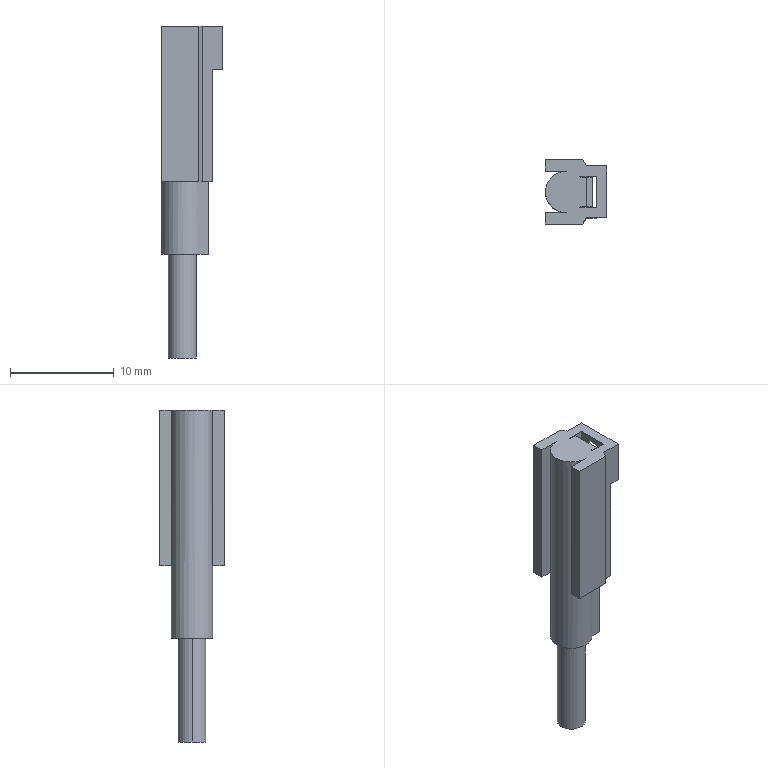Part | SolidWorks | features ICE 8, RefAxis 3, 3DProfileFeature 1, Extrusion 1 | 1 solid | 51 faces | box 5.9 x 6.2 x 32 mm | volume 553.468 mm3 | plane 37 | cylinder 14 | commonest cylinder face diameters 0.8 x4 2.1 x3 2.5 x2 2.7 x2 2.9 x2 4 x1
STEP:
#1=CARTESIAN_POINT('',(1.35,0.,-32.));
#2=VERTEX_POINT('',#1);
#3=CARTESIAN_POINT('',(-1.35,0.,-32.));
#4=VERTEX_POINT('',#3);
#5=CARTESIAN_POINT('',(0.,0.,-32.));
#6=DIRECTION('',(0.,0.,1.));
#7=DIRECTION('',(1.,0.,0.));
#8=AXIS2_PLACEMENT_3D('',#5,#6,#7);
#9=CIRCLE('',#8,1.35);
#10=EDGE_CURVE('',#2,#4,#9,.T.);
#11=ORIENTED_EDGE('',*,*,#10,.T.);
#12=CARTESIAN_POINT('',(-1.35,0.,-22.));
#13=VERTEX_POINT('',#12);
#14=CARTESIAN_POINT('',(-1.35,0.,-32.));
#15=DIRECTION('',(0.,0.,1.));
#16=VECTOR('',#15,1000.);
#17=LINE('',#14,#16);
#18=EDGE_CURVE('',#4,#13,#17,.T.);
#19=ORIENTED_EDGE('',*,*,#18,.T.);
#20=CARTESIAN_POINT('',(1.35,0.,-22.));
#21=VERTEX_POINT('',#20);
#22=CARTESIAN_POINT('',(0.,0.,-22.));
#23=DIRECTION('',(0.,0.,1.));
#24=DIRECTION('',(1.,0.,0.));
#25=AXIS2_PLACEMENT_3D('',#22,#23,#24);
#26=CIRCLE('',#25,1.35);
#27=EDGE_CURVE('',#21,#13,#26,.T.);
#28=ORIENTED_EDGE('',*,*,#27,.F.);
#29=CARTESIAN_POINT('',(1.35,0.,-32.));
#30=DIRECTION('',(0.,0.,1.));
#31=VECTOR('',#30,1000.);
#32=LINE('',#29,#31);
#33=EDGE_CURVE('',#2,#21,#32,.T.);
#34=ORIENTED_EDGE('',*,*,#33,.F.);
#35=EDGE_LOOP('',(#11,#19,#28,#34));
#36=FACE_OUTER_BOUND('',#35,.T.);
#37=CARTESIAN_POINT('',(0.,0.,-32.));
#38=DIRECTION('',(0.,0.,1.));
#39=DIRECTION('',(1.,0.,0.));
#40=AXIS2_PLACEMENT_3D('',#37,#38,#39);
#41=CYLINDRICAL_SURFACE('',#40,1.35);
#42=ADVANCED_FACE('',(#36),#41,.T.);
#43=CARTESIAN_POINT('',(1.9,0.,-0.75));
#44=VERTEX_POINT('',#43);
#45=CARTESIAN_POINT('',(1.9,0.,-3.25));
#46=VERTEX_POINT('',#45);
#47=CARTESIAN_POINT('',(1.9,0.,-2.));
#48=DIRECTION('',(1.,0.,0.));
#49=DIRECTION('',(0.,0.,-1.));
#50=AXIS2_PLACEMENT_3D('',#47,#48,#49);
#51=CIRCLE('',#50,1.25);
#52=EDGE_CURVE('',#44,#46,#51,.T.);
#53=ORIENTED_EDGE('',*,*,#52,.F.);
#54=CARTESIAN_POINT('',(2.,0.,-0.75));
#55=VERTEX_POINT('',#54);
#56=CARTESIAN_POINT('',(1.9,0.,-0.75));
#57=DIRECTION('',(1.,0.,0.));
#58=VECTOR('',#57,1000.);
#59=LINE('',#56,#58);
#60=EDGE_CURVE('',#44,#55,#59,.T.);
#61=ORIENTED_EDGE('',*,*,#60,.T.);
#62=CARTESIAN_POINT('',(2.,0.,-3.25));
#63=VERTEX_POINT('',#62);
#64=CARTESIAN_POINT('',(2.,0.,-2.));
#65=DIRECTION('',(1.,0.,0.));
#66=DIRECTION('',(0.,0.,-1.));
#67=AXIS2_PLACEMENT_3D('',#64,#65,#66);
#68=CIRCLE('',#67,1.25);
#69=EDGE_CURVE('',#55,#63,#68,.T.);
#70=ORIENTED_EDGE('',*,*,#69,.T.);
#71=CARTESIAN_POINT('',(1.9,0.,-3.25));
#72=DIRECTION('',(1.,0.,0.));
#73=VECTOR('',#72,1000.);
#74=LINE('',#71,#73);
#75=EDGE_CURVE('',#46,#63,#74,.T.);
#76=ORIENTED_EDGE('',*,*,#75,.F.);
#77=EDGE_LOOP('',(#53,#61,#70,#76));
#78=FACE_OUTER_BOUND('',#77,.T.);
#79=CARTESIAN_POINT('',(1.9,0.,-2.));
#80=DIRECTION('',(1.,0.,0.));
#81=DIRECTION('',(0.,0.,-1.));
#82=AXIS2_PLACEMENT_3D('',#79,#80,#81);
#83=CYLINDRICAL_SURFACE('',#82,1.25);
#84=ADVANCED_FACE('',(#78),#83,.F.);
#85=CARTESIAN_POINT('',(2.9,0.,-0.55));
#86=VERTEX_POINT('',#85);
#87=CARTESIAN_POINT('',(2.9,0.,-3.45));
#88=VERTEX_POINT('',#87);
#89=CARTESIAN_POINT('',(2.9,0.,-2.));
#90=DIRECTION('',(1.,0.,0.));
#91=DIRECTION('',(0.,0.,-1.));
#92=AXIS2_PLACEMENT_3D('',#89,#90,#91);
#93=CIRCLE('',#92,1.45);
#94=EDGE_CURVE('',#86,#88,#93,.T.);
#95=ORIENTED_EDGE('',*,*,#94,.F.);
#96=CARTESIAN_POINT('',(3.9,0.,-0.55));
#97=VERTEX_POINT('',#96);
#98=CARTESIAN_POINT('',(2.9,0.,-0.55));
#99=DIRECTION('',(1.,0.,0.));
#100=VECTOR('',#99,1000.);
#101=LINE('',#98,#100);
#102=EDGE_CURVE('',#86,#97,#101,.T.);
#103=ORIENTED_EDGE('',*,*,#102,.T.);
#104=CARTESIAN_POINT('',(3.9,0.,-3.45));
#105=VERTEX_POINT('',#104);
#106=CARTESIAN_POINT('',(3.9,0.,-2.));
#107=DIRECTION('',(1.,0.,0.));
#108=DIRECTION('',(0.,0.,-1.));
#109=AXIS2_PLACEMENT_3D('',#106,#107,#108);
#110=CIRCLE('',#109,1.45);
#111=EDGE_CURVE('',#97,#105,#110,.T.);
#112=ORIENTED_EDGE('',*,*,#111,.T.);
#113=CARTESIAN_POINT('',(2.9,0.,-3.45));
#114=DIRECTION('',(1.,0.,0.));
#115=VECTOR('',#114,1000.);
#116=LINE('',#113,#115);
#117=EDGE_CURVE('',#88,#105,#116,.T.);
#118=ORIENTED_EDGE('',*,*,#117,.F.);
#119=EDGE_LOOP('',(#95,#103,#112,#118));
#120=FACE_OUTER_BOUND('',#119,.T.);
#121=CARTESIAN_POINT('',(2.9,0.,-2.));
#122=DIRECTION('',(1.,0.,0.));
#123=DIRECTION('',(0.,0.,-1.));
#124=AXIS2_PLACEMENT_3D('',#121,#122,#123);
#125=CYLINDRICAL_SURFACE('',#124,1.45);
#126=ADVANCED_FACE('',(#120),#125,.F.);
#127=CARTESIAN_POINT('',(1.9,-0.4994,-2.924));
#128=VERTEX_POINT('',#127);
#129=CARTESIAN_POINT('',(1.9,0.,-3.05));
#130=VERTEX_POINT('',#129);
#131=CARTESIAN_POINT('',(1.9,0.,-2.));
#132=DIRECTION('',(1.,0.,0.));
#133=DIRECTION('',(0.,0.,-1.));
#134=AXIS2_PLACEMENT_3D('',#131,#132,#133);
#135=CIRCLE('',#134,1.05);
#136=EDGE_CURVE('',#128,#130,#135,.T.);
#137=ORIENTED_EDGE('',*,*,#136,.T.);
#138=CARTESIAN_POINT('',(2.,0.,-3.05));
#139=VERTEX_POINT('',#138);
#140=CARTESIAN_POINT('',(1.9,0.,-3.05));
#141=DIRECTION('',(1.,0.,0.));
#142=VECTOR('',#141,1000.);
#143=LINE('',#140,#142);
#144=EDGE_CURVE('',#130,#139,#143,.T.);
#145=ORIENTED_EDGE('',*,*,#144,.T.);
#146=CARTESIAN_POINT('',(2.,-0.4994,-2.924));
#147=VERTEX_POINT('',#146);
#148=CARTESIAN_POINT('',(2.,0.,-2.));
#149=DIRECTION('',(1.,0.,0.));
#150=DIRECTION('',(0.,0.,-1.));
#151=AXIS2_PLACEMENT_3D('',#148,#149,#150);
#152=CIRCLE('',#151,1.05);
#153=EDGE_CURVE('',#147,#139,#152,.T.);
#154=ORIENTED_EDGE('',*,*,#153,.F.);
#155=CARTESIAN_POINT('',(1.9,-0.4994,-2.924));
#156=DIRECTION('',(1.,0.,0.));
#157=VECTOR('',#156,1000.);
#158=LINE('',#155,#157);
#159=EDGE_CURVE('',#128,#147,#158,.T.);
#160=ORIENTED_EDGE('',*,*,#159,.F.);
#161=EDGE_LOOP('',(#137,#145,#154,#160));
#162=FACE_OUTER_BOUND('',#161,.T.);
#163=CARTESIAN_POINT('',(1.9,0.,-2.));
#164=DIRECTION('',(1.,0.,0.));
#165=DIRECTION('',(0.,0.,-1.));
#166=AXIS2_PLACEMENT_3D('',#163,#164,#165);
#167=CYLINDRICAL_SURFACE('',#166,1.05);
#168=ADVANCED_FACE('',(#162),#167,.T.);
#169=ORIENTED_EDGE('',*,*,#144,.F.);
#170=CARTESIAN_POINT('',(1.9,0.9236,-1.501));
#171=VERTEX_POINT('',#170);
#172=CARTESIAN_POINT('',(1.9,0.,-2.));
#173=DIRECTION('',(1.,0.,0.));
#174=DIRECTION('',(0.,0.,-1.));
#175=AXIS2_PLACEMENT_3D('',#172,#173,#174);
#176=CIRCLE('',#175,1.05);
#177=EDGE_CURVE('',#130,#171,#176,.T.);
#178=ORIENTED_EDGE('',*,*,#177,.T.);
#179=CARTESIAN_POINT('',(2.,0.9236,-1.501));
#180=VERTEX_POINT('',#179);
#181=CARTESIAN_POINT('',(1.9,0.9236,-1.501));
#182=DIRECTION('',(-1.,0.,0.));
#183=VECTOR('',#182,1000.);
#184=LINE('',#181,#183);
#185=EDGE_CURVE('',#180,#171,#184,.T.);
#186=ORIENTED_EDGE('',*,*,#185,.F.);
#187=CARTESIAN_POINT('',(2.,0.,-2.));
#188=DIRECTION('',(1.,0.,0.));
#189=DIRECTION('',(0.,0.,-1.));
#190=AXIS2_PLACEMENT_3D('',#187,#188,#189);
#191=CIRCLE('',#190,1.05);
#192=EDGE_CURVE('',#139,#180,#191,.T.);
#193=ORIENTED_EDGE('',*,*,#192,.F.);
#194=EDGE_LOOP('',(#169,#178,#186,#193));
#195=FACE_OUTER_BOUND('',#194,.T.);
#196=CARTESIAN_POINT('',(1.9,0.,-2.));
#197=DIRECTION('',(1.,0.,0.));
#198=DIRECTION('',(0.,0.,-1.));
#199=AXIS2_PLACEMENT_3D('',#196,#197,#198);
#200=CYLINDRICAL_SURFACE('',#199,1.05);
#201=ADVANCED_FACE('',(#195),#200,.T.);
#202=ORIENTED_EDGE('',*,*,#153,.T.);
#203=ORIENTED_EDGE('',*,*,#192,.T.);
#204=CARTESIAN_POINT('',(2.,-1.988,-4.412));
#205=DIRECTION('',(0.,-0.7071,-0.7071));
#206=VECTOR('',#205,1000.);
#207=LINE('',#204,#206);
#208=EDGE_CURVE('',#180,#147,#207,.T.);
#209=ORIENTED_EDGE('',*,*,#208,.T.);
#210=EDGE_LOOP('',(#202,#203,#209));
#211=FACE_OUTER_BOUND('',#210,.T.);
#212=CARTESIAN_POINT('',(2.,-1.4,-5.));
#213=DIRECTION('',(-1.,0.,0.));
#214=DIRECTION('',(0.,0.,1.));
#215=AXIS2_PLACEMENT_3D('',#212,#213,#214);
#216=PLANE('',#215);
#217=ADVANCED_FACE('',(#211),#216,.F.);
#218=CARTESIAN_POINT('',(2.9,-2.5,-15.));
#219=VERTEX_POINT('',#218);
#220=CARTESIAN_POINT('',(2.9,-1.5,-15.));
#221=VERTEX_POINT('',#220);
#222=CARTESIAN_POINT('',(2.9,0.,-15.));
#223=DIRECTION('',(0.,1.,0.));
#224=VECTOR('',#223,1000.);
#225=LINE('',#222,#224);
#226=EDGE_CURVE('',#219,#221,#225,.T.);
#227=ORIENTED_EDGE('',*,*,#226,.F.);
#228=CARTESIAN_POINT('',(1.946,-2.5,-15.));
#229=VERTEX_POINT('',#228);
#230=CARTESIAN_POINT('',(1.946,-2.5,-15.));
#231=DIRECTION('',(1.,0.,0.));
#232=VECTOR('',#231,1000.);
#233=LINE('',#230,#232);
#234=EDGE_CURVE('',#229,#219,#233,.T.);
#235=ORIENTED_EDGE('',*,*,#234,.F.);
#236=CARTESIAN_POINT('',(1.6,-3.1,-15.));
#237=VERTEX_POINT('',#236);
#238=CARTESIAN_POINT('',(1.6,-3.1,-15.));
#239=DIRECTION('',(0.5,0.866,0.));
#240=VECTOR('',#239,1000.);
#241=LINE('',#238,#240);
#242=EDGE_CURVE('',#237,#229,#241,.T.);
#243=ORIENTED_EDGE('',*,*,#242,.F.);
#244=CARTESIAN_POINT('',(-2.,-3.1,-15.));
#245=VERTEX_POINT('',#244);
#246=CARTESIAN_POINT('',(-2.,-3.1,-15.));
#247=DIRECTION('',(1.,0.,0.));
#248=VECTOR('',#247,1000.);
#249=LINE('',#246,#248);
#250=EDGE_CURVE('',#245,#237,#249,.T.);
#251=ORIENTED_EDGE('',*,*,#250,.F.);
#252=CARTESIAN_POINT('',(-2.,-2.,-15.));
#253=VERTEX_POINT('',#252);
#254=CARTESIAN_POINT('',(-2.,-2.,-15.));
#255=DIRECTION('',(0.,-1.,0.));
#256=VECTOR('',#255,1000.);
#257=LINE('',#254,#256);
#258=EDGE_CURVE('',#253,#245,#257,.T.);
#259=ORIENTED_EDGE('',*,*,#258,.F.);
#260=CARTESIAN_POINT('',(0.,-2.,-15.));
#261=VERTEX_POINT('',#260);
#262=CARTESIAN_POINT('',(0.,-2.,-15.));
#263=DIRECTION('',(-1.,0.,0.));
#264=VECTOR('',#263,1000.);
#265=LINE('',#262,#264);
#266=EDGE_CURVE('',#261,#253,#265,.T.);
#267=ORIENTED_EDGE('',*,*,#266,.F.);
#268=CARTESIAN_POINT('',(1.323,-1.5,-15.));
#269=VERTEX_POINT('',#268);
#270=CARTESIAN_POINT('',(0.,0.,-15.));
#271=DIRECTION('',(0.,0.,-1.));
#272=DIRECTION('',(-1.,0.,0.));
#273=AXIS2_PLACEMENT_3D('',#270,#271,#272);
#274=CIRCLE('',#273,2.);
#275=EDGE_CURVE('',#269,#261,#274,.T.);
#276=ORIENTED_EDGE('',*,*,#275,.F.);
#277=CARTESIAN_POINT('',(2.9,-1.5,-15.));
#278=DIRECTION('',(-1.,0.,0.));
#279=VECTOR('',#278,1000.);
#280=LINE('',#277,#279);
#281=EDGE_CURVE('',#221,#269,#280,.T.);
#282=ORIENTED_EDGE('',*,*,#281,.F.);
#283=EDGE_LOOP('',(#227,#235,#243,#251,#259,#267,#276,#282));
#284=FACE_OUTER_BOUND('',#283,.T.);
#285=CARTESIAN_POINT('',(0.,0.,-15.));
#286=DIRECTION('',(0.,0.,-1.));
#287=DIRECTION('',(-1.,0.,0.));
#288=AXIS2_PLACEMENT_3D('',#285,#286,#287);
#289=PLANE('',#288);
#290=ADVANCED_FACE('',(#284),#289,.T.);
#291=CARTESIAN_POINT('',(-2.,-2.,0.));
#292=VERTEX_POINT('',#291);
#293=CARTESIAN_POINT('',(-2.,-3.1,0.));
#294=VERTEX_POINT('',#293);
#295=CARTESIAN_POINT('',(-2.,-2.,0.));
#296=DIRECTION('',(0.,-1.,0.));
#297=VECTOR('',#296,1000.);
#298=LINE('',#295,#297);
#299=EDGE_CURVE('',#292,#294,#298,.T.);
#300=ORIENTED_EDGE('',*,*,#299,.F.);
#301=CARTESIAN_POINT('',(-2.,-2.,-15.));
#302=DIRECTION('',(0.,0.,1.));
#303=VECTOR('',#302,1000.);
#304=LINE('',#301,#303);
#305=EDGE_CURVE('',#253,#292,#304,.T.);
#306=ORIENTED_EDGE('',*,*,#305,.F.);
#307=ORIENTED_EDGE('',*,*,#258,.T.);
#308=CARTESIAN_POINT('',(-2.,-3.1,-15.));
#309=DIRECTION('',(0.,0.,1.));
#310=VECTOR('',#309,1000.);
#311=LINE('',#308,#310);
#312=EDGE_CURVE('',#245,#294,#311,.T.);
#313=ORIENTED_EDGE('',*,*,#312,.T.);
#314=EDGE_LOOP('',(#300,#306,#307,#313));
#315=FACE_OUTER_BOUND('',#314,.T.);
#316=CARTESIAN_POINT('',(-2.,-2.,-15.));
#317=DIRECTION('',(-1.,0.,0.));
#318=DIRECTION('',(0.,0.,1.));
#319=AXIS2_PLACEMENT_3D('',#316,#317,#318);
#320=PLANE('',#319);
#321=ADVANCED_FACE('',(#315),#320,.T.);
#322=CARTESIAN_POINT('',(0.,-2.,0.));
#323=VERTEX_POINT('',#322);
#324=CARTESIAN_POINT('',(0.,-2.,0.));
#325=DIRECTION('',(-1.,0.,0.));
#326=VECTOR('',#325,1000.);
#327=LINE('',#324,#326);
#328=EDGE_CURVE('',#323,#292,#327,.T.);
#329=ORIENTED_EDGE('',*,*,#328,.F.);
#330=CARTESIAN_POINT('',(0.,-2.,-15.));
#331=DIRECTION('',(0.,0.,1.));
#332=VECTOR('',#331,1000.);
#333=LINE('',#330,#332);
#334=EDGE_CURVE('',#261,#323,#333,.T.);
#335=ORIENTED_EDGE('',*,*,#334,.F.);
#336=ORIENTED_EDGE('',*,*,#266,.T.);
#337=ORIENTED_EDGE('',*,*,#305,.T.);
#338=EDGE_LOOP('',(#329,#335,#336,#337));
#339=FACE_OUTER_BOUND('',#338,.T.);
#340=CARTESIAN_POINT('',(0.,-2.,-15.));
#341=DIRECTION('',(0.,1.,0.));
#342=DIRECTION('',(0.,0.,1.));
#343=AXIS2_PLACEMENT_3D('',#340,#341,#342);
#344=PLANE('',#343);
#345=ADVANCED_FACE('',(#339),#344,.T.);
#346=CARTESIAN_POINT('',(2.9,-1.5,0.));
#347=VERTEX_POINT('',#346);
#348=CARTESIAN_POINT('',(1.323,-1.5,0.));
#349=VERTEX_POINT('',#348);
#350=CARTESIAN_POINT('',(2.9,-1.5,0.));
#351=DIRECTION('',(-1.,0.,0.));
#352=VECTOR('',#351,1000.);
#353=LINE('',#350,#352);
#354=EDGE_CURVE('',#347,#349,#353,.T.);
#355=ORIENTED_EDGE('',*,*,#354,.F.);
#356=CARTESIAN_POINT('',(2.9,-1.5,-4.2));
#357=VERTEX_POINT('',#356);
#358=CARTESIAN_POINT('',(2.9,-1.5,-15.));
#359=DIRECTION('',(0.,0.,1.));
#360=VECTOR('',#359,1000.);
#361=LINE('',#358,#360);
#362=EDGE_CURVE('',#357,#347,#361,.T.);
#363=ORIENTED_EDGE('',*,*,#362,.F.);
#364=CARTESIAN_POINT('',(2.9,-1.5,-15.));
#365=DIRECTION('',(0.,0.,1.));
#366=VECTOR('',#365,1000.);
#367=LINE('',#364,#366);
#368=EDGE_CURVE('',#221,#357,#367,.T.);
#369=ORIENTED_EDGE('',*,*,#368,.F.);
#370=ORIENTED_EDGE('',*,*,#281,.T.);
#371=CARTESIAN_POINT('',(1.323,-1.5,-15.));
#372=DIRECTION('',(0.,0.,1.));
#373=VECTOR('',#372,1000.);
#374=LINE('',#371,#373);
#375=EDGE_CURVE('',#269,#349,#374,.T.);
#376=ORIENTED_EDGE('',*,*,#375,.T.);
#377=EDGE_LOOP('',(#355,#363,#369,#370,#376));
#378=FACE_OUTER_BOUND('',#377,.T.);
#379=CARTESIAN_POINT('',(2.9,-1.5,-15.));
#380=DIRECTION('',(0.,1.,0.));
#381=DIRECTION('',(0.,0.,1.));
#382=AXIS2_PLACEMENT_3D('',#379,#380,#381);
#383=PLANE('',#382);
#384=ADVANCED_FACE('',(#378),#383,.T.);
#385=CARTESIAN_POINT('',(2.9,0.,-2.));
#386=DIRECTION('',(1.,0.,0.));
#387=DIRECTION('',(0.,0.,-1.));
#388=AXIS2_PLACEMENT_3D('',#385,#386,#387);
#389=CIRCLE('',#388,1.45);
#390=EDGE_CURVE('',#88,#86,#389,.T.);
#391=ORIENTED_EDGE('',*,*,#390,.T.);
#392=ORIENTED_EDGE('',*,*,#94,.T.);
#393=EDGE_LOOP('',(#391,#392));
#394=FACE_BOUND('',#393,.T.);
#395=CARTESIAN_POINT('',(2.9,1.5,-4.2));
#396=VERTEX_POINT('',#395);
#397=CARTESIAN_POINT('',(2.9,2.5,-4.2));
#398=DIRECTION('',(0.,-1.,0.));
#399=VECTOR('',#398,1000.);
#400=LINE('',#397,#399);
#401=EDGE_CURVE('',#396,#357,#400,.T.);
#402=ORIENTED_EDGE('',*,*,#401,.T.);
#403=ORIENTED_EDGE('',*,*,#362,.T.);
#404=CARTESIAN_POINT('',(2.9,1.5,0.));
#405=VERTEX_POINT('',#404);
#406=CARTESIAN_POINT('',(2.9,1.5,0.));
#407=DIRECTION('',(0.,-1.,0.));
#408=VECTOR('',#407,1000.);
#409=LINE('',#406,#408);
#410=EDGE_CURVE('',#405,#347,#409,.T.);
#411=ORIENTED_EDGE('',*,*,#410,.F.);
#412=CARTESIAN_POINT('',(2.9,1.5,-15.));
#413=DIRECTION('',(0.,0.,1.));
#414=VECTOR('',#413,1000.);
#415=LINE('',#412,#414);
#416=EDGE_CURVE('',#396,#405,#415,.T.);
#417=ORIENTED_EDGE('',*,*,#416,.F.);
#418=EDGE_LOOP('',(#402,#403,#411,#417));
#419=FACE_OUTER_BOUND('',#418,.T.);
#420=CARTESIAN_POINT('',(2.9,1.5,-15.));
#421=DIRECTION('',(-1.,0.,0.));
#422=DIRECTION('',(0.,0.,1.));
#423=AXIS2_PLACEMENT_3D('',#420,#421,#422);
#424=PLANE('',#423);
#425=ADVANCED_FACE('',(#394,#419),#424,.T.);
#426=CARTESIAN_POINT('',(1.323,1.5,0.));
#427=VERTEX_POINT('',#426);
#428=CARTESIAN_POINT('',(1.323,1.5,0.));
#429=DIRECTION('',(1.,0.,0.));
#430=VECTOR('',#429,1000.);
#431=LINE('',#428,#430);
#432=EDGE_CURVE('',#427,#405,#431,.T.);
#433=ORIENTED_EDGE('',*,*,#432,.F.);
#434=CARTESIAN_POINT('',(1.323,1.5,-15.));
#435=VERTEX_POINT('',#434);
#436=CARTESIAN_POINT('',(1.323,1.5,-15.));
#437=DIRECTION('',(0.,0.,1.));
#438=VECTOR('',#437,1000.);
#439=LINE('',#436,#438);
#440=EDGE_CURVE('',#435,#427,#439,.T.);
#441=ORIENTED_EDGE('',*,*,#440,.F.);
#442=CARTESIAN_POINT('',(2.9,1.5,-15.));
#443=VERTEX_POINT('',#442);
#444=CARTESIAN_POINT('',(1.323,1.5,-15.));
#445=DIRECTION('',(1.,0.,0.));
#446=VECTOR('',#445,1000.);
#447=LINE('',#444,#446);
#448=EDGE_CURVE('',#435,#443,#447,.T.);
#449=ORIENTED_EDGE('',*,*,#448,.T.);
#450=CARTESIAN_POINT('',(2.9,1.5,-15.));
#451=DIRECTION('',(0.,0.,1.));
#452=VECTOR('',#451,1000.);
#453=LINE('',#450,#452);
#454=EDGE_CURVE('',#443,#396,#453,.T.);
#455=ORIENTED_EDGE('',*,*,#454,.T.);
#456=ORIENTED_EDGE('',*,*,#416,.T.);
#457=EDGE_LOOP('',(#433,#441,#449,#455,#456));
#458=FACE_OUTER_BOUND('',#457,.T.);
#459=CARTESIAN_POINT('',(1.323,1.5,-15.));
#460=DIRECTION('',(0.,-1.,0.));
#461=DIRECTION('',(0.,0.,-1.));
#462=AXIS2_PLACEMENT_3D('',#459,#460,#461);
#463=PLANE('',#462);
#464=ADVANCED_FACE('',(#458),#463,.T.);
#465=CARTESIAN_POINT('',(-2.,2.,0.));
#466=VERTEX_POINT('',#465);
#467=CARTESIAN_POINT('',(0.,2.,0.));
#468=VERTEX_POINT('',#467);
#469=CARTESIAN_POINT('',(-2.,2.,0.));
#470=DIRECTION('',(1.,0.,0.));
#471=VECTOR('',#470,1000.);
#472=LINE('',#469,#471);
#473=EDGE_CURVE('',#466,#468,#472,.T.);
#474=ORIENTED_EDGE('',*,*,#473,.F.);
#475=CARTESIAN_POINT('',(-2.,2.,-15.));
#476=VERTEX_POINT('',#475);
#477=CARTESIAN_POINT('',(-2.,2.,-15.));
#478=DIRECTION('',(0.,0.,1.));
#479=VECTOR('',#478,1000.);
#480=LINE('',#477,#479);
#481=EDGE_CURVE('',#476,#466,#480,.T.);
#482=ORIENTED_EDGE('',*,*,#481,.F.);
#483=CARTESIAN_POINT('',(0.,2.,-15.));
#484=VERTEX_POINT('',#483);
#485=CARTESIAN_POINT('',(-2.,2.,-15.));
#486=DIRECTION('',(1.,0.,0.));
#487=VECTOR('',#486,1000.);
#488=LINE('',#485,#487);
#489=EDGE_CURVE('',#476,#484,#488,.T.);
#490=ORIENTED_EDGE('',*,*,#489,.T.);
#491=CARTESIAN_POINT('',(0.,2.,-15.));
#492=DIRECTION('',(0.,0.,1.));
#493=VECTOR('',#492,1000.);
#494=LINE('',#491,#493);
#495=EDGE_CURVE('',#484,#468,#494,.T.);
#496=ORIENTED_EDGE('',*,*,#495,.T.);
#497=EDGE_LOOP('',(#474,#482,#490,#496));
#498=FACE_OUTER_BOUND('',#497,.T.);
#499=CARTESIAN_POINT('',(-2.,2.,-15.));
#500=DIRECTION('',(0.,-1.,0.));
#501=DIRECTION('',(0.,0.,-1.));
#502=AXIS2_PLACEMENT_3D('',#499,#500,#501);
#503=PLANE('',#502);
#504=ADVANCED_FACE('',(#498),#503,.T.);
#505=CARTESIAN_POINT('',(-2.,3.1,0.));
#506=VERTEX_POINT('',#505);
#507=CARTESIAN_POINT('',(-2.,3.1,0.));
#508=DIRECTION('',(0.,-1.,0.));
#509=VECTOR('',#508,1000.);
#510=LINE('',#507,#509);
#511=EDGE_CURVE('',#506,#466,#510,.T.);
#512=ORIENTED_EDGE('',*,*,#511,.F.);
#513=CARTESIAN_POINT('',(-2.,3.1,-15.));
#514=VERTEX_POINT('',#513);
#515=CARTESIAN_POINT('',(-2.,3.1,-15.));
#516=DIRECTION('',(0.,0.,1.));
#517=VECTOR('',#516,1000.);
#518=LINE('',#515,#517);
#519=EDGE_CURVE('',#514,#506,#518,.T.);
#520=ORIENTED_EDGE('',*,*,#519,.F.);
#521=CARTESIAN_POINT('',(-2.,3.1,-15.));
#522=DIRECTION('',(0.,-1.,0.));
#523=VECTOR('',#522,1000.);
#524=LINE('',#521,#523);
#525=EDGE_CURVE('',#514,#476,#524,.T.);
#526=ORIENTED_EDGE('',*,*,#525,.T.);
#527=ORIENTED_EDGE('',*,*,#481,.T.);
#528=EDGE_LOOP('',(#512,#520,#526,#527));
#529=FACE_OUTER_BOUND('',#528,.T.);
#530=CARTESIAN_POINT('',(-2.,3.1,-15.));
#531=DIRECTION('',(-1.,0.,0.));
#532=DIRECTION('',(0.,0.,1.));
#533=AXIS2_PLACEMENT_3D('',#530,#531,#532);
#534=PLANE('',#533);
#535=ADVANCED_FACE('',(#529),#534,.T.);
#536=CARTESIAN_POINT('',(1.6,3.1,0.));
#537=VERTEX_POINT('',#536);
#538=CARTESIAN_POINT('',(1.6,3.1,0.));
#539=DIRECTION('',(-1.,0.,0.));
#540=VECTOR('',#539,1000.);
#541=LINE('',#538,#540);
#542=EDGE_CURVE('',#537,#506,#541,.T.);
#543=ORIENTED_EDGE('',*,*,#542,.F.);
#544=CARTESIAN_POINT('',(1.6,3.1,-15.));
#545=VERTEX_POINT('',#544);
#546=CARTESIAN_POINT('',(1.6,3.1,-15.));
#547=DIRECTION('',(0.,0.,1.));
#548=VECTOR('',#547,1000.);
#549=LINE('',#546,#548);
#550=EDGE_CURVE('',#545,#537,#549,.T.);
#551=ORIENTED_EDGE('',*,*,#550,.F.);
#552=CARTESIAN_POINT('',(1.6,3.1,-15.));
#553=DIRECTION('',(-1.,0.,0.));
#554=VECTOR('',#553,1000.);
#555=LINE('',#552,#554);
#556=EDGE_CURVE('',#545,#514,#555,.T.);
#557=ORIENTED_EDGE('',*,*,#556,.T.);
#558=ORIENTED_EDGE('',*,*,#519,.T.);
#559=EDGE_LOOP('',(#543,#551,#557,#558));
#560=FACE_OUTER_BOUND('',#559,.T.);
#561=CARTESIAN_POINT('',(1.6,3.1,-15.));
#562=DIRECTION('',(0.,1.,0.));
#563=DIRECTION('',(0.,0.,1.));
#564=AXIS2_PLACEMENT_3D('',#561,#562,#563);
#565=PLANE('',#564);
#566=ADVANCED_FACE('',(#560),#565,.T.);
#567=CARTESIAN_POINT('',(1.946,2.5,0.));
#568=VERTEX_POINT('',#567);
#569=CARTESIAN_POINT('',(1.946,2.5,0.));
#570=DIRECTION('',(-0.5,0.866,0.));
#571=VECTOR('',#570,1000.);
#572=LINE('',#569,#571);
#573=EDGE_CURVE('',#568,#537,#572,.T.);
#574=ORIENTED_EDGE('',*,*,#573,.F.);
#575=CARTESIAN_POINT('',(1.946,2.5,-15.));
#576=VERTEX_POINT('',#575);
#577=CARTESIAN_POINT('',(1.946,2.5,-15.));
#578=DIRECTION('',(0.,0.,1.));
#579=VECTOR('',#578,1000.);
#580=LINE('',#577,#579);
#581=EDGE_CURVE('',#576,#568,#580,.T.);
#582=ORIENTED_EDGE('',*,*,#581,.F.);
#583=CARTESIAN_POINT('',(1.946,2.5,-15.));
#584=DIRECTION('',(-0.5,0.866,0.));
#585=VECTOR('',#584,1000.);
#586=LINE('',#583,#585);
#587=EDGE_CURVE('',#576,#545,#586,.T.);
#588=ORIENTED_EDGE('',*,*,#587,.T.);
#589=ORIENTED_EDGE('',*,*,#550,.T.);
#590=EDGE_LOOP('',(#574,#582,#588,#589));
#591=FACE_OUTER_BOUND('',#590,.T.);
#592=CARTESIAN_POINT('',(1.946,2.5,-15.));
#593=DIRECTION('',(0.866,0.5,0.));
#594=DIRECTION('',(-0.5,0.866,0.));
#595=AXIS2_PLACEMENT_3D('',#592,#593,#594);
#596=PLANE('',#595);
#597=ADVANCED_FACE('',(#591),#596,.T.);
#598=CARTESIAN_POINT('',(2.9,2.5,-15.));
#599=VERTEX_POINT('',#598);
#600=CARTESIAN_POINT('',(2.9,2.5,-4.2));
#601=VERTEX_POINT('',#600);
#602=CARTESIAN_POINT('',(2.9,2.5,-15.));
#603=DIRECTION('',(0.,0.,1.));
#604=VECTOR('',#603,1000.);
#605=LINE('',#602,#604);
#606=EDGE_CURVE('',#599,#601,#605,.T.);
#607=ORIENTED_EDGE('',*,*,#606,.F.);
#608=CARTESIAN_POINT('',(3.9,2.5,-15.));
#609=DIRECTION('',(-1.,0.,0.));
#610=VECTOR('',#609,1000.);
#611=LINE('',#608,#610);
#612=EDGE_CURVE('',#599,#576,#611,.T.);
#613=ORIENTED_EDGE('',*,*,#612,.T.);
#614=ORIENTED_EDGE('',*,*,#581,.T.);
#615=CARTESIAN_POINT('',(3.9,2.5,0.));
#616=VERTEX_POINT('',#615);
#617=CARTESIAN_POINT('',(3.9,2.5,0.));
#618=DIRECTION('',(-1.,0.,0.));
#619=VECTOR('',#618,1000.);
#620=LINE('',#617,#619);
#621=EDGE_CURVE('',#616,#568,#620,.T.);
#622=ORIENTED_EDGE('',*,*,#621,.F.);
#623=CARTESIAN_POINT('',(3.9,2.5,-4.2));
#624=VERTEX_POINT('',#623);
#625=CARTESIAN_POINT('',(3.9,2.5,-15.));
#626=DIRECTION('',(0.,0.,1.));
#627=VECTOR('',#626,1000.);
#628=LINE('',#625,#627);
#629=EDGE_CURVE('',#624,#616,#628,.T.);
#630=ORIENTED_EDGE('',*,*,#629,.F.);
#631=CARTESIAN_POINT('',(3.9,2.5,-4.2));
#632=DIRECTION('',(-1.,0.,0.));
#633=VECTOR('',#632,1000.);
#634=LINE('',#631,#633);
#635=EDGE_CURVE('',#624,#601,#634,.T.);
#636=ORIENTED_EDGE('',*,*,#635,.T.);
#637=EDGE_LOOP('',(#607,#613,#614,#622,#630,#636));
#638=FACE_OUTER_BOUND('',#637,.T.);
#639=CARTESIAN_POINT('',(3.9,2.5,-15.));
#640=DIRECTION('',(0.,1.,0.));
#641=DIRECTION('',(0.,0.,1.));
#642=AXIS2_PLACEMENT_3D('',#639,#640,#641);
#643=PLANE('',#642);
#644=ADVANCED_FACE('',(#638),#643,.T.);
#645=CARTESIAN_POINT('',(3.9,0.,-2.));
#646=DIRECTION('',(1.,0.,0.));
#647=DIRECTION('',(0.,0.,-1.));
#648=AXIS2_PLACEMENT_3D('',#645,#646,#647);
#649=CIRCLE('',#648,1.45);
#650=EDGE_CURVE('',#105,#97,#649,.T.);
#651=ORIENTED_EDGE('',*,*,#650,.F.);
#652=ORIENTED_EDGE('',*,*,#111,.F.);
#653=EDGE_LOOP('',(#651,#652));
#654=FACE_BOUND('',#653,.T.);
#655=CARTESIAN_POINT('',(3.9,-2.5,-4.2));
#656=VERTEX_POINT('',#655);
#657=CARTESIAN_POINT('',(3.9,-2.5,-4.2));
#658=DIRECTION('',(0.,1.,0.));
#659=VECTOR('',#658,1000.);
#660=LINE('',#657,#659);
#661=EDGE_CURVE('',#656,#624,#660,.T.);
#662=ORIENTED_EDGE('',*,*,#661,.T.);
#663=ORIENTED_EDGE('',*,*,#629,.T.);
#664=CARTESIAN_POINT('',(3.9,-2.5,0.));
#665=VERTEX_POINT('',#664);
#666=CARTESIAN_POINT('',(3.9,-2.5,0.));
#667=DIRECTION('',(0.,1.,0.));
#668=VECTOR('',#667,1000.);
#669=LINE('',#666,#668);
#670=EDGE_CURVE('',#665,#616,#669,.T.);
#671=ORIENTED_EDGE('',*,*,#670,.F.);
#672=CARTESIAN_POINT('',(3.9,-2.5,-15.));
#673=DIRECTION('',(0.,0.,1.));
#674=VECTOR('',#673,1000.);
#675=LINE('',#672,#674);
#676=EDGE_CURVE('',#656,#665,#675,.T.);
#677=ORIENTED_EDGE('',*,*,#676,.F.);
#678=EDGE_LOOP('',(#662,#663,#671,#677));
#679=FACE_OUTER_BOUND('',#678,.T.);
#680=CARTESIAN_POINT('',(3.9,-2.5,-15.));
#681=DIRECTION('',(1.,0.,0.));
#682=DIRECTION('',(0.,0.,-1.));
#683=AXIS2_PLACEMENT_3D('',#680,#681,#682);
#684=PLANE('',#683);
#685=ADVANCED_FACE('',(#654,#679),#684,.T.);
#686=CARTESIAN_POINT('',(2.9,-2.5,-4.2));
#687=VERTEX_POINT('',#686);
#688=CARTESIAN_POINT('',(2.9,-2.5,-15.));
#689=DIRECTION('',(0.,0.,1.));
#690=VECTOR('',#689,1000.);
#691=LINE('',#688,#690);
#692=EDGE_CURVE('',#219,#687,#691,.T.);
#693=ORIENTED_EDGE('',*,*,#692,.T.);
#694=CARTESIAN_POINT('',(2.9,-2.5,-4.2));
#695=DIRECTION('',(1.,0.,0.));
#696=VECTOR('',#695,1000.);
#697=LINE('',#694,#696);
#698=EDGE_CURVE('',#687,#656,#697,.T.);
#699=ORIENTED_EDGE('',*,*,#698,.T.);
#700=ORIENTED_EDGE('',*,*,#676,.T.);
#701=CARTESIAN_POINT('',(1.946,-2.5,0.));
#702=VERTEX_POINT('',#701);
#703=CARTESIAN_POINT('',(1.946,-2.5,0.));
#704=DIRECTION('',(1.,0.,0.));
#705=VECTOR('',#704,1000.);
#706=LINE('',#703,#705);
#707=EDGE_CURVE('',#702,#665,#706,.T.);
#708=ORIENTED_EDGE('',*,*,#707,.F.);
#709=CARTESIAN_POINT('',(1.946,-2.5,-15.));
#710=DIRECTION('',(0.,0.,1.));
#711=VECTOR('',#710,1000.);
#712=LINE('',#709,#711);
#713=EDGE_CURVE('',#229,#702,#712,.T.);
#714=ORIENTED_EDGE('',*,*,#713,.F.);
#715=ORIENTED_EDGE('',*,*,#234,.T.);
#716=EDGE_LOOP('',(#693,#699,#700,#708,#714,#715));
#717=FACE_OUTER_BOUND('',#716,.T.);
#718=CARTESIAN_POINT('',(1.946,-2.5,-15.));
#719=DIRECTION('',(0.,-1.,0.));
#720=DIRECTION('',(0.,0.,-1.));
#721=AXIS2_PLACEMENT_3D('',#718,#719,#720);
#722=PLANE('',#721);
#723=ADVANCED_FACE('',(#717),#722,.T.);
#724=CARTESIAN_POINT('',(1.6,-3.1,0.));
#725=VERTEX_POINT('',#724);
#726=CARTESIAN_POINT('',(1.6,-3.1,0.));
#727=DIRECTION('',(0.5,0.866,0.));
#728=VECTOR('',#727,1000.);
#729=LINE('',#726,#728);
#730=EDGE_CURVE('',#725,#702,#729,.T.);
#731=ORIENTED_EDGE('',*,*,#730,.F.);
#732=CARTESIAN_POINT('',(1.6,-3.1,-15.));
#733=DIRECTION('',(0.,0.,1.));
#734=VECTOR('',#733,1000.);
#735=LINE('',#732,#734);
#736=EDGE_CURVE('',#237,#725,#735,.T.);
#737=ORIENTED_EDGE('',*,*,#736,.F.);
#738=ORIENTED_EDGE('',*,*,#242,.T.);
#739=ORIENTED_EDGE('',*,*,#713,.T.);
#740=EDGE_LOOP('',(#731,#737,#738,#739));
#741=FACE_OUTER_BOUND('',#740,.T.);
#742=CARTESIAN_POINT('',(1.6,-3.1,-15.));
#743=DIRECTION('',(0.866,-0.5,0.));
#744=DIRECTION('',(0.5,0.866,0.));
#745=AXIS2_PLACEMENT_3D('',#742,#743,#744);
#746=PLANE('',#745);
#747=ADVANCED_FACE('',(#741),#746,.T.);
#748=CARTESIAN_POINT('',(-2.,-3.1,0.));
#749=DIRECTION('',(1.,0.,0.));
#750=VECTOR('',#749,1000.);
#751=LINE('',#748,#750);
#752=EDGE_CURVE('',#294,#725,#751,.T.);
#753=ORIENTED_EDGE('',*,*,#752,.F.);
#754=ORIENTED_EDGE('',*,*,#312,.F.);
#755=ORIENTED_EDGE('',*,*,#250,.T.);
#756=ORIENTED_EDGE('',*,*,#736,.T.);
#757=EDGE_LOOP('',(#753,#754,#755,#756));
#758=FACE_OUTER_BOUND('',#757,.T.);
#759=CARTESIAN_POINT('',(-2.,-3.1,-15.));
#760=DIRECTION('',(0.,-1.,0.));
#761=DIRECTION('',(0.,0.,-1.));
#762=AXIS2_PLACEMENT_3D('',#759,#760,#761);
#763=PLANE('',#762);
#764=ADVANCED_FACE('',(#758),#763,.T.);
#765=CARTESIAN_POINT('',(2.9,2.5,-15.));
#766=DIRECTION('',(0.,-1.,0.));
#767=VECTOR('',#766,1000.);
#768=LINE('',#765,#767);
#769=EDGE_CURVE('',#599,#443,#768,.T.);
#770=ORIENTED_EDGE('',*,*,#769,.T.);
#771=ORIENTED_EDGE('',*,*,#448,.F.);
#772=CARTESIAN_POINT('',(0.,0.,-15.));
#773=DIRECTION('',(0.,0.,-1.));
#774=DIRECTION('',(-1.,0.,0.));
#775=AXIS2_PLACEMENT_3D('',#772,#773,#774);
#776=CIRCLE('',#775,2.);
#777=EDGE_CURVE('',#484,#435,#776,.T.);
#778=ORIENTED_EDGE('',*,*,#777,.F.);
#779=ORIENTED_EDGE('',*,*,#489,.F.);
#780=ORIENTED_EDGE('',*,*,#525,.F.);
#781=ORIENTED_EDGE('',*,*,#556,.F.);
#782=ORIENTED_EDGE('',*,*,#587,.F.);
#783=ORIENTED_EDGE('',*,*,#612,.F.);
#784=EDGE_LOOP('',(#770,#771,#778,#779,#780,#781,#782,#783));
#785=FACE_OUTER_BOUND('',#784,.T.);
#786=CARTESIAN_POINT('',(0.,0.,-15.));
#787=DIRECTION('',(0.,0.,-1.));
#788=DIRECTION('',(-1.,0.,0.));
#789=AXIS2_PLACEMENT_3D('',#786,#787,#788);
#790=PLANE('',#789);
#791=ADVANCED_FACE('',(#785),#790,.T.);
#792=CARTESIAN_POINT('',(1.428,-1.4,0.));
#793=VERTEX_POINT('',#792);
#794=CARTESIAN_POINT('',(2.,-1.4,0.));
#795=VERTEX_POINT('',#794);
#796=CARTESIAN_POINT('',(1.428,-1.4,0.));
#797=DIRECTION('',(1.,0.,0.));
#798=VECTOR('',#797,1000.);
#799=LINE('',#796,#798);
#800=EDGE_CURVE('',#793,#795,#799,.T.);
#801=ORIENTED_EDGE('',*,*,#800,.T.);
#802=CARTESIAN_POINT('',(2.,1.4,0.));
#803=VERTEX_POINT('',#802);
#804=CARTESIAN_POINT('',(2.,-1.4,0.));
#805=DIRECTION('',(0.,1.,0.));
#806=VECTOR('',#805,1000.);
#807=LINE('',#804,#806);
#808=EDGE_CURVE('',#795,#803,#807,.T.);
#809=ORIENTED_EDGE('',*,*,#808,.T.);
#810=CARTESIAN_POINT('',(1.428,1.4,0.));
#811=VERTEX_POINT('',#810);
#812=CARTESIAN_POINT('',(2.5,1.4,0.));
#813=DIRECTION('',(-1.,0.,0.));
#814=VECTOR('',#813,1000.);
#815=LINE('',#812,#814);
#816=EDGE_CURVE('',#803,#811,#815,.T.);
#817=ORIENTED_EDGE('',*,*,#816,.T.);
#818=CARTESIAN_POINT('',(0.,0.,0.));
#819=DIRECTION('',(0.,0.,1.));
#820=DIRECTION('',(1.,0.,0.));
#821=AXIS2_PLACEMENT_3D('',#818,#819,#820);
#822=CIRCLE('',#821,2.);
#823=EDGE_CURVE('',#811,#427,#822,.T.);
#824=ORIENTED_EDGE('',*,*,#823,.T.);
#825=ORIENTED_EDGE('',*,*,#432,.T.);
#826=ORIENTED_EDGE('',*,*,#410,.T.);
#827=ORIENTED_EDGE('',*,*,#354,.T.);
#828=CARTESIAN_POINT('',(0.,0.,0.));
#829=DIRECTION('',(0.,0.,1.));
#830=DIRECTION('',(1.,0.,0.));
#831=AXIS2_PLACEMENT_3D('',#828,#829,#830);
#832=CIRCLE('',#831,2.);
#833=EDGE_CURVE('',#349,#793,#832,.T.);
#834=ORIENTED_EDGE('',*,*,#833,.T.);
#835=EDGE_LOOP('',(#801,#809,#817,#824,#825,#826,#827,#834));
#836=FACE_BOUND('',#835,.T.);
#837=ORIENTED_EDGE('',*,*,#299,.T.);
#838=ORIENTED_EDGE('',*,*,#752,.T.);
#839=ORIENTED_EDGE('',*,*,#730,.T.);
#840=ORIENTED_EDGE('',*,*,#707,.T.);
#841=ORIENTED_EDGE('',*,*,#670,.T.);
#842=ORIENTED_EDGE('',*,*,#621,.T.);
#843=ORIENTED_EDGE('',*,*,#573,.T.);
#844=ORIENTED_EDGE('',*,*,#542,.T.);
#845=ORIENTED_EDGE('',*,*,#511,.T.);
#846=ORIENTED_EDGE('',*,*,#473,.T.);
#847=CARTESIAN_POINT('',(0.,0.,0.));
#848=DIRECTION('',(0.,0.,1.));
#849=DIRECTION('',(1.,0.,0.));
#850=AXIS2_PLACEMENT_3D('',#847,#848,#849);
#851=CIRCLE('',#850,2.);
#852=EDGE_CURVE('',#468,#323,#851,.T.);
#853=ORIENTED_EDGE('',*,*,#852,.T.);
#854=ORIENTED_EDGE('',*,*,#328,.T.);
#855=EDGE_LOOP('',(#837,#838,#839,#840,#841,#842,#843,#844,#845,#846,#853,#854));
#856=FACE_OUTER_BOUND('',#855,.T.);
#857=CARTESIAN_POINT('',(0.,0.,0.));
#858=DIRECTION('',(0.,0.,-1.));
#859=DIRECTION('',(-1.,0.,0.));
#860=AXIS2_PLACEMENT_3D('',#857,#858,#859);
#861=PLANE('',#860);
#862=ADVANCED_FACE('',(#836,#856),#861,.F.);
#863=ORIENTED_EDGE('',*,*,#368,.T.);
#864=CARTESIAN_POINT('',(2.9,2.5,-4.2));
#865=DIRECTION('',(0.,-1.,0.));
#866=VECTOR('',#865,1000.);
#867=LINE('',#864,#866);
#868=EDGE_CURVE('',#357,#687,#867,.T.);
#869=ORIENTED_EDGE('',*,*,#868,.T.);
#870=ORIENTED_EDGE('',*,*,#692,.F.);
#871=ORIENTED_EDGE('',*,*,#226,.T.);
#872=EDGE_LOOP('',(#863,#869,#870,#871));
#873=FACE_OUTER_BOUND('',#872,.T.);
#874=CARTESIAN_POINT('',(2.9,2.5,-15.));
#875=DIRECTION('',(-1.,0.,0.));
#876=DIRECTION('',(0.,0.,1.));
#877=AXIS2_PLACEMENT_3D('',#874,#875,#876);
#878=PLANE('',#877);
#879=ADVANCED_FACE('',(#873),#878,.F.);
#880=ORIENTED_EDGE('',*,*,#454,.F.);
#881=ORIENTED_EDGE('',*,*,#769,.F.);
#882=ORIENTED_EDGE('',*,*,#606,.T.);
#883=CARTESIAN_POINT('',(2.9,2.5,-4.2));
#884=DIRECTION('',(0.,-1.,0.));
#885=VECTOR('',#884,1000.);
#886=LINE('',#883,#885);
#887=EDGE_CURVE('',#601,#396,#886,.T.);
#888=ORIENTED_EDGE('',*,*,#887,.T.);
#889=EDGE_LOOP('',(#880,#881,#882,#888));
#890=FACE_OUTER_BOUND('',#889,.T.);
#891=CARTESIAN_POINT('',(2.9,2.5,-15.));
#892=DIRECTION('',(-1.,0.,0.));
#893=DIRECTION('',(0.,0.,1.));
#894=AXIS2_PLACEMENT_3D('',#891,#892,#893);
#895=PLANE('',#894);
#896=ADVANCED_FACE('',(#890),#895,.F.);
#897=ORIENTED_EDGE('',*,*,#887,.F.);
#898=ORIENTED_EDGE('',*,*,#635,.F.);
#899=ORIENTED_EDGE('',*,*,#661,.F.);
#900=ORIENTED_EDGE('',*,*,#698,.F.);
#901=ORIENTED_EDGE('',*,*,#868,.F.);
#902=ORIENTED_EDGE('',*,*,#401,.F.);
#903=EDGE_LOOP('',(#897,#898,#899,#900,#901,#902));
#904=FACE_OUTER_BOUND('',#903,.T.);
#905=CARTESIAN_POINT('',(0.,0.,-4.2));
#906=DIRECTION('',(0.,0.,1.));
#907=DIRECTION('',(1.,0.,0.));
#908=AXIS2_PLACEMENT_3D('',#905,#906,#907);
#909=PLANE('',#908);
#910=ADVANCED_FACE('',(#904),#909,.F.);
#911=ORIENTED_EDGE('',*,*,#102,.F.);
#912=ORIENTED_EDGE('',*,*,#390,.F.);
#913=ORIENTED_EDGE('',*,*,#117,.T.);
#914=ORIENTED_EDGE('',*,*,#650,.T.);
#915=EDGE_LOOP('',(#911,#912,#913,#914));
#916=FACE_OUTER_BOUND('',#915,.T.);
#917=CARTESIAN_POINT('',(2.9,0.,-2.));
#918=DIRECTION('',(1.,0.,0.));
#919=DIRECTION('',(0.,0.,-1.));
#920=AXIS2_PLACEMENT_3D('',#917,#918,#919);
#921=CYLINDRICAL_SURFACE('',#920,1.45);
#922=ADVANCED_FACE('',(#916),#921,.F.);
#923=ORIENTED_EDGE('',*,*,#275,.T.);
#924=ORIENTED_EDGE('',*,*,#334,.T.);
#925=ORIENTED_EDGE('',*,*,#852,.F.);
#926=ORIENTED_EDGE('',*,*,#495,.F.);
#927=ORIENTED_EDGE('',*,*,#777,.T.);
#928=ORIENTED_EDGE('',*,*,#440,.T.);
#929=ORIENTED_EDGE('',*,*,#823,.F.);
#930=CARTESIAN_POINT('',(1.428,1.4,-22.));
#931=VERTEX_POINT('',#930);
#932=CARTESIAN_POINT('',(1.428,1.4,-22.));
#933=DIRECTION('',(0.,0.,1.));
#934=VECTOR('',#933,1000.);
#935=LINE('',#932,#934);
#936=EDGE_CURVE('',#931,#811,#935,.T.);
#937=ORIENTED_EDGE('',*,*,#936,.F.);
#938=CARTESIAN_POINT('',(1.428,-1.4,-22.));
#939=VERTEX_POINT('',#938);
#940=CARTESIAN_POINT('',(0.,0.,-22.));
#941=DIRECTION('',(0.,0.,1.));
#942=DIRECTION('',(1.,0.,0.));
#943=AXIS2_PLACEMENT_3D('',#940,#941,#942);
#944=CIRCLE('',#943,2.);
#945=EDGE_CURVE('',#931,#939,#944,.T.);
#946=ORIENTED_EDGE('',*,*,#945,.T.);
#947=CARTESIAN_POINT('',(1.428,-1.4,-22.));
#948=DIRECTION('',(0.,0.,1.));
#949=VECTOR('',#948,1000.);
#950=LINE('',#947,#949);
#951=EDGE_CURVE('',#939,#793,#950,.T.);
#952=ORIENTED_EDGE('',*,*,#951,.T.);
#953=ORIENTED_EDGE('',*,*,#833,.F.);
#954=ORIENTED_EDGE('',*,*,#375,.F.);
#955=EDGE_LOOP('',(#923,#924,#925,#926,#927,#928,#929,#937,#946,#952,#953,#954));
#956=FACE_OUTER_BOUND('',#955,.T.);
#957=CARTESIAN_POINT('',(0.,0.,-22.));
#958=DIRECTION('',(0.,0.,1.));
#959=DIRECTION('',(1.,0.,0.));
#960=AXIS2_PLACEMENT_3D('',#957,#958,#959);
#961=CYLINDRICAL_SURFACE('',#960,2.);
#962=ADVANCED_FACE('',(#956),#961,.T.);
#963=CARTESIAN_POINT('',(2.,1.4,-5.));
#964=VERTEX_POINT('',#963);
#965=CARTESIAN_POINT('',(2.,1.4,-5.));
#966=DIRECTION('',(0.,0.,1.));
#967=VECTOR('',#966,1000.);
#968=LINE('',#965,#967);
#969=EDGE_CURVE('',#964,#803,#968,.T.);
#970=ORIENTED_EDGE('',*,*,#969,.F.);
#971=CARTESIAN_POINT('',(2.5,1.4,-5.));
#972=VERTEX_POINT('',#971);
#973=CARTESIAN_POINT('',(2.5,1.4,-5.));
#974=DIRECTION('',(-1.,0.,0.));
#975=VECTOR('',#974,1000.);
#976=LINE('',#973,#975);
#977=EDGE_CURVE('',#972,#964,#976,.T.);
#978=ORIENTED_EDGE('',*,*,#977,.F.);
#979=CARTESIAN_POINT('',(2.5,1.4,-22.));
#980=VERTEX_POINT('',#979);
#981=CARTESIAN_POINT('',(2.5,1.4,-22.));
#982=DIRECTION('',(0.,0.,1.));
#983=VECTOR('',#982,1000.);
#984=LINE('',#981,#983);
#985=EDGE_CURVE('',#980,#972,#984,.T.);
#986=ORIENTED_EDGE('',*,*,#985,.F.);
#987=CARTESIAN_POINT('',(2.5,1.4,-22.));
#988=DIRECTION('',(-1.,0.,0.));
#989=VECTOR('',#988,1000.);
#990=LINE('',#987,#989);
#991=EDGE_CURVE('',#980,#931,#990,.T.);
#992=ORIENTED_EDGE('',*,*,#991,.T.);
#993=ORIENTED_EDGE('',*,*,#936,.T.);
#994=ORIENTED_EDGE('',*,*,#816,.F.);
#995=EDGE_LOOP('',(#970,#978,#986,#992,#993,#994));
#996=FACE_OUTER_BOUND('',#995,.T.);
#997=CARTESIAN_POINT('',(2.5,1.4,-22.));
#998=DIRECTION('',(0.,1.,0.));
#999=DIRECTION('',(0.,0.,1.));
#1000=AXIS2_PLACEMENT_3D('',#997,#998,#999);
#1001=PLANE('',#1000);
#1002=ADVANCED_FACE('',(#996),#1001,.T.);
#1003=CARTESIAN_POINT('',(2.5,-0.4,-7.));
#1004=VERTEX_POINT('',#1003);
#1005=CARTESIAN_POINT('',(2.5,-0.8,-7.4));
#1006=VERTEX_POINT('',#1005);
#1007=CARTESIAN_POINT('',(2.5,-0.4,-7.4));
#1008=DIRECTION('',(1.,0.,0.));
#1009=DIRECTION('',(0.,0.,-1.));
#1010=AXIS2_PLACEMENT_3D('',#1007,#1008,#1009);
#1011=CIRCLE('',#1010,0.4);
#1012=EDGE_CURVE('',#1004,#1006,#1011,.T.);
#1013=ORIENTED_EDGE('',*,*,#1012,.F.);
#1014=CARTESIAN_POINT('',(2.5,0.4,-7.));
#1015=VERTEX_POINT('',#1014);
#1016=CARTESIAN_POINT('',(2.5,0.4,-7.));
#1017=DIRECTION('',(0.,-1.,0.));
#1018=VECTOR('',#1017,1000.);
#1019=LINE('',#1016,#1018);
#1020=EDGE_CURVE('',#1015,#1004,#1019,.T.);
#1021=ORIENTED_EDGE('',*,*,#1020,.F.);
#1022=CARTESIAN_POINT('',(2.5,0.8,-7.4));
#1023=VERTEX_POINT('',#1022);
#1024=CARTESIAN_POINT('',(2.5,0.4,-7.4));
#1025=DIRECTION('',(1.,0.,0.));
#1026=DIRECTION('',(0.,0.,-1.));
#1027=AXIS2_PLACEMENT_3D('',#1024,#1025,#1026);
#1028=CIRCLE('',#1027,0.4);
#1029=EDGE_CURVE('',#1023,#1015,#1028,.T.);
#1030=ORIENTED_EDGE('',*,*,#1029,.F.);
#1031=CARTESIAN_POINT('',(2.5,0.8,-9.6));
#1032=VERTEX_POINT('',#1031);
#1033=CARTESIAN_POINT('',(2.5,0.8,-9.6));
#1034=DIRECTION('',(0.,0.,1.));
#1035=VECTOR('',#1034,1000.);
#1036=LINE('',#1033,#1035);
#1037=EDGE_CURVE('',#1032,#1023,#1036,.T.);
#1038=ORIENTED_EDGE('',*,*,#1037,.F.);
#1039=CARTESIAN_POINT('',(2.5,0.4,-10.));
#1040=VERTEX_POINT('',#1039);
#1041=CARTESIAN_POINT('',(2.5,0.4,-9.6));
#1042=DIRECTION('',(1.,0.,0.));
#1043=DIRECTION('',(0.,0.,-1.));
#1044=AXIS2_PLACEMENT_3D('',#1041,#1042,#1043);
#1045=CIRCLE('',#1044,0.4);
#1046=EDGE_CURVE('',#1040,#1032,#1045,.T.);
#1047=ORIENTED_EDGE('',*,*,#1046,.F.);
#1048=CARTESIAN_POINT('',(2.5,-0.4,-10.));
#1049=VERTEX_POINT('',#1048);
#1050=CARTESIAN_POINT('',(2.5,-0.4,-10.));
#1051=DIRECTION('',(0.,1.,0.));
#1052=VECTOR('',#1051,1000.);
#1053=LINE('',#1050,#1052);
#1054=EDGE_CURVE('',#1049,#1040,#1053,.T.);
#1055=ORIENTED_EDGE('',*,*,#1054,.F.);
#1056=CARTESIAN_POINT('',(2.5,-0.8,-9.6));
#1057=VERTEX_POINT('',#1056);
#1058=CARTESIAN_POINT('',(2.5,-0.4,-9.6));
#1059=DIRECTION('',(1.,0.,0.));
#1060=DIRECTION('',(0.,0.,-1.));
#1061=AXIS2_PLACEMENT_3D('',#1058,#1059,#1060);
#1062=CIRCLE('',#1061,0.4);
#1063=EDGE_CURVE('',#1057,#1049,#1062,.T.);
#1064=ORIENTED_EDGE('',*,*,#1063,.F.);
#1065=CARTESIAN_POINT('',(2.5,-0.8,-7.4));
#1066=DIRECTION('',(0.,0.,-1.));
#1067=VECTOR('',#1066,1000.);
#1068=LINE('',#1065,#1067);
#1069=EDGE_CURVE('',#1006,#1057,#1068,.T.);
#1070=ORIENTED_EDGE('',*,*,#1069,.F.);
#1071=EDGE_LOOP('',(#1013,#1021,#1030,#1038,#1047,#1055,#1064,#1070));
#1072=FACE_BOUND('',#1071,.T.);
#1073=CARTESIAN_POINT('',(2.5,-1.4,-5.));
#1074=VERTEX_POINT('',#1073);
#1075=CARTESIAN_POINT('',(2.5,-1.4,-5.));
#1076=DIRECTION('',(0.,1.,0.));
#1077=VECTOR('',#1076,1000.);
#1078=LINE('',#1075,#1077);
#1079=EDGE_CURVE('',#1074,#972,#1078,.T.);
#1080=ORIENTED_EDGE('',*,*,#1079,.F.);
#1081=CARTESIAN_POINT('',(2.5,-1.4,-22.));
#1082=VERTEX_POINT('',#1081);
#1083=CARTESIAN_POINT('',(2.5,-1.4,-22.));
#1084=DIRECTION('',(0.,0.,1.));
#1085=VECTOR('',#1084,1000.);
#1086=LINE('',#1083,#1085);
#1087=EDGE_CURVE('',#1082,#1074,#1086,.T.);
#1088=ORIENTED_EDGE('',*,*,#1087,.F.);
#1089=CARTESIAN_POINT('',(2.5,-1.4,-22.));
#1090=DIRECTION('',(0.,1.,0.));
#1091=VECTOR('',#1090,1000.);
#1092=LINE('',#1089,#1091);
#1093=EDGE_CURVE('',#1082,#980,#1092,.T.);
#1094=ORIENTED_EDGE('',*,*,#1093,.T.);
#1095=ORIENTED_EDGE('',*,*,#985,.T.);
#1096=EDGE_LOOP('',(#1080,#1088,#1094,#1095));
#1097=FACE_OUTER_BOUND('',#1096,.T.);
#1098=CARTESIAN_POINT('',(2.5,-1.4,-22.));
#1099=DIRECTION('',(1.,0.,0.));
#1100=DIRECTION('',(0.,0.,-1.));
#1101=AXIS2_PLACEMENT_3D('',#1098,#1099,#1100);
#1102=PLANE('',#1101);
#1103=ADVANCED_FACE('',(#1072,#1097),#1102,.T.);
#1104=CARTESIAN_POINT('',(2.,-1.4,-5.));
#1105=VERTEX_POINT('',#1104);
#1106=CARTESIAN_POINT('',(2.,-1.4,-5.));
#1107=DIRECTION('',(0.,0.,1.));
#1108=VECTOR('',#1107,1000.);
#1109=LINE('',#1106,#1108);
#1110=EDGE_CURVE('',#1105,#795,#1109,.T.);
#1111=ORIENTED_EDGE('',*,*,#1110,.T.);
#1112=ORIENTED_EDGE('',*,*,#800,.F.);
#1113=ORIENTED_EDGE('',*,*,#951,.F.);
#1114=CARTESIAN_POINT('',(1.428,-1.4,-22.));
#1115=DIRECTION('',(1.,0.,0.));
#1116=VECTOR('',#1115,1000.);
#1117=LINE('',#1114,#1116);
#1118=EDGE_CURVE('',#939,#1082,#1117,.T.);
#1119=ORIENTED_EDGE('',*,*,#1118,.T.);
#1120=ORIENTED_EDGE('',*,*,#1087,.T.);
#1121=CARTESIAN_POINT('',(2.5,-1.4,-5.));
#1122=DIRECTION('',(-1.,0.,0.));
#1123=VECTOR('',#1122,1000.);
#1124=LINE('',#1121,#1123);
#1125=EDGE_CURVE('',#1074,#1105,#1124,.T.);
#1126=ORIENTED_EDGE('',*,*,#1125,.T.);
#1127=EDGE_LOOP('',(#1111,#1112,#1113,#1119,#1120,#1126));
#1128=FACE_OUTER_BOUND('',#1127,.T.);
#1129=CARTESIAN_POINT('',(1.428,-1.4,-22.));
#1130=DIRECTION('',(0.,-1.,0.));
#1131=DIRECTION('',(0.,0.,-1.));
#1132=AXIS2_PLACEMENT_3D('',#1129,#1130,#1131);
#1133=PLANE('',#1132);
#1134=ADVANCED_FACE('',(#1128),#1133,.T.);
#1135=ORIENTED_EDGE('',*,*,#27,.T.);
#1136=CARTESIAN_POINT('',(0.,0.,-22.));
#1137=DIRECTION('',(0.,0.,1.));
#1138=DIRECTION('',(1.,0.,0.));
#1139=AXIS2_PLACEMENT_3D('',#1136,#1137,#1138);
#1140=CIRCLE('',#1139,1.35);
#1141=EDGE_CURVE('',#13,#21,#1140,.T.);
#1142=ORIENTED_EDGE('',*,*,#1141,.T.);
#1143=EDGE_LOOP('',(#1135,#1142));
#1144=FACE_BOUND('',#1143,.T.);
#1145=ORIENTED_EDGE('',*,*,#945,.F.);
#1146=ORIENTED_EDGE('',*,*,#991,.F.);
#1147=ORIENTED_EDGE('',*,*,#1093,.F.);
#1148=ORIENTED_EDGE('',*,*,#1118,.F.);
#1149=EDGE_LOOP('',(#1145,#1146,#1147,#1148));
#1150=FACE_OUTER_BOUND('',#1149,.T.);
#1151=CARTESIAN_POINT('',(0.,0.,-22.));
#1152=DIRECTION('',(0.,0.,1.));
#1153=DIRECTION('',(1.,0.,0.));
#1154=AXIS2_PLACEMENT_3D('',#1151,#1152,#1153);
#1155=PLANE('',#1154);
#1156=ADVANCED_FACE('',(#1144,#1150),#1155,.F.);
#1157=CARTESIAN_POINT('',(2.,0.,-2.));
#1158=DIRECTION('',(1.,0.,0.));
#1159=DIRECTION('',(0.,0.,-1.));
#1160=AXIS2_PLACEMENT_3D('',#1157,#1158,#1159);
#1161=CIRCLE('',#1160,1.25);
#1162=EDGE_CURVE('',#63,#55,#1161,.T.);
#1163=ORIENTED_EDGE('',*,*,#1162,.F.);
#1164=ORIENTED_EDGE('',*,*,#69,.F.);
#1165=EDGE_LOOP('',(#1163,#1164));
#1166=FACE_BOUND('',#1165,.T.);
#1167=ORIENTED_EDGE('',*,*,#808,.F.);
#1168=ORIENTED_EDGE('',*,*,#1110,.F.);
#1169=CARTESIAN_POINT('',(2.,-1.4,-5.));
#1170=DIRECTION('',(0.,1.,0.));
#1171=VECTOR('',#1170,1000.);
#1172=LINE('',#1169,#1171);
#1173=EDGE_CURVE('',#1105,#964,#1172,.T.);
#1174=ORIENTED_EDGE('',*,*,#1173,.T.);
#1175=ORIENTED_EDGE('',*,*,#969,.T.);
#1176=EDGE_LOOP('',(#1167,#1168,#1174,#1175));
#1177=FACE_OUTER_BOUND('',#1176,.T.);
#1178=CARTESIAN_POINT('',(2.,-1.4,-5.));
#1179=DIRECTION('',(-1.,0.,0.));
#1180=DIRECTION('',(0.,0.,1.));
#1181=AXIS2_PLACEMENT_3D('',#1178,#1179,#1180);
#1182=PLANE('',#1181);
#1183=ADVANCED_FACE('',(#1166,#1177),#1182,.F.);
#1184=ORIENTED_EDGE('',*,*,#1173,.F.);
#1185=ORIENTED_EDGE('',*,*,#1125,.F.);
#1186=ORIENTED_EDGE('',*,*,#1079,.T.);
#1187=ORIENTED_EDGE('',*,*,#977,.T.);
#1188=EDGE_LOOP('',(#1184,#1185,#1186,#1187));
#1189=FACE_OUTER_BOUND('',#1188,.T.);
#1190=CARTESIAN_POINT('',(2.5,-1.4,-5.));
#1191=DIRECTION('',(0.,0.,-1.));
#1192=DIRECTION('',(-1.,0.,0.));
#1193=AXIS2_PLACEMENT_3D('',#1190,#1191,#1192);
#1194=PLANE('',#1193);
#1195=ADVANCED_FACE('',(#1189),#1194,.F.);
#1196=ORIENTED_EDGE('',*,*,#60,.F.);
#1197=CARTESIAN_POINT('',(1.9,0.,-2.));
#1198=DIRECTION('',(1.,0.,0.));
#1199=DIRECTION('',(0.,0.,-1.));
#1200=AXIS2_PLACEMENT_3D('',#1197,#1198,#1199);
#1201=CIRCLE('',#1200,1.25);
#1202=EDGE_CURVE('',#46,#44,#1201,.T.);
#1203=ORIENTED_EDGE('',*,*,#1202,.F.);
#1204=ORIENTED_EDGE('',*,*,#75,.T.);
#1205=ORIENTED_EDGE('',*,*,#1162,.T.);
#1206=EDGE_LOOP('',(#1196,#1203,#1204,#1205));
#1207=FACE_OUTER_BOUND('',#1206,.T.);
#1208=CARTESIAN_POINT('',(1.9,0.,-2.));
#1209=DIRECTION('',(1.,0.,0.));
#1210=DIRECTION('',(0.,0.,-1.));
#1211=AXIS2_PLACEMENT_3D('',#1208,#1209,#1210);
#1212=CYLINDRICAL_SURFACE('',#1211,1.25);
#1213=ADVANCED_FACE('',(#1207),#1212,.F.);
#1214=ORIENTED_EDGE('',*,*,#136,.F.);
#1215=CARTESIAN_POINT('',(1.9,-0.6095,-3.034));
#1216=DIRECTION('',(0.,0.7071,0.7071));
#1217=VECTOR('',#1216,1000.);
#1218=LINE('',#1215,#1217);
#1219=EDGE_CURVE('',#128,#171,#1218,.T.);
#1220=ORIENTED_EDGE('',*,*,#1219,.T.);
#1221=ORIENTED_EDGE('',*,*,#177,.F.);
#1222=EDGE_LOOP('',(#1214,#1220,#1221));
#1223=FACE_BOUND('',#1222,.T.);
#1224=CARTESIAN_POINT('',(1.9,0.4994,-1.076));
#1225=VERTEX_POINT('',#1224);
#1226=CARTESIAN_POINT('',(1.9,-0.9236,-2.499));
#1227=VERTEX_POINT('',#1226);
#1228=CARTESIAN_POINT('',(1.9,0.,-2.));
#1229=DIRECTION('',(1.,0.,0.));
#1230=DIRECTION('',(0.,0.,-1.));
#1231=AXIS2_PLACEMENT_3D('',#1228,#1229,#1230);
#1232=CIRCLE('',#1231,1.05);
#1233=EDGE_CURVE('',#1225,#1227,#1232,.T.);
#1234=ORIENTED_EDGE('',*,*,#1233,.F.);
#1235=CARTESIAN_POINT('',(1.9,0.6095,-0.9663));
#1236=DIRECTION('',(0.,-0.7071,-0.7071));
#1237=VECTOR('',#1236,1000.);
#1238=LINE('',#1235,#1237);
#1239=EDGE_CURVE('',#1225,#1227,#1238,.T.);
#1240=ORIENTED_EDGE('',*,*,#1239,.T.);
#1241=EDGE_LOOP('',(#1234,#1240));
#1242=FACE_BOUND('',#1241,.T.);
#1243=ORIENTED_EDGE('',*,*,#1202,.T.);
#1244=ORIENTED_EDGE('',*,*,#52,.T.);
#1245=EDGE_LOOP('',(#1243,#1244));
#1246=FACE_OUTER_BOUND('',#1245,.T.);
#1247=CARTESIAN_POINT('',(1.9,0.,-2.));
#1248=DIRECTION('',(1.,0.,0.));
#1249=DIRECTION('',(0.,0.,-1.));
#1250=AXIS2_PLACEMENT_3D('',#1247,#1248,#1249);
#1251=PLANE('',#1250);
#1252=ADVANCED_FACE('',(#1223,#1242,#1246),#1251,.T.);
#1253=CARTESIAN_POINT('',(2.,-0.9236,-2.499));
#1254=VERTEX_POINT('',#1253);
#1255=CARTESIAN_POINT('',(1.9,-0.9236,-2.499));
#1256=DIRECTION('',(-1.,0.,0.));
#1257=VECTOR('',#1256,1000.);
#1258=LINE('',#1255,#1257);
#1259=EDGE_CURVE('',#1254,#1227,#1258,.T.);
#1260=ORIENTED_EDGE('',*,*,#1259,.F.);
#1261=CARTESIAN_POINT('',(2.,0.4994,-1.076));
#1262=VERTEX_POINT('',#1261);
#1263=CARTESIAN_POINT('',(2.,0.,-2.));
#1264=DIRECTION('',(1.,0.,0.));
#1265=DIRECTION('',(0.,0.,-1.));
#1266=AXIS2_PLACEMENT_3D('',#1263,#1264,#1265);
#1267=CIRCLE('',#1266,1.05);
#1268=EDGE_CURVE('',#1262,#1254,#1267,.T.);
#1269=ORIENTED_EDGE('',*,*,#1268,.F.);
#1270=CARTESIAN_POINT('',(1.9,0.4994,-1.076));
#1271=DIRECTION('',(1.,0.,0.));
#1272=VECTOR('',#1271,1000.);
#1273=LINE('',#1270,#1272);
#1274=EDGE_CURVE('',#1225,#1262,#1273,.T.);
#1275=ORIENTED_EDGE('',*,*,#1274,.F.);
#1276=ORIENTED_EDGE('',*,*,#1233,.T.);
#1277=EDGE_LOOP('',(#1260,#1269,#1275,#1276));
#1278=FACE_OUTER_BOUND('',#1277,.T.);
#1279=CARTESIAN_POINT('',(1.9,0.,-2.));
#1280=DIRECTION('',(1.,0.,0.));
#1281=DIRECTION('',(0.,0.,-1.));
#1282=AXIS2_PLACEMENT_3D('',#1279,#1280,#1281);
#1283=CYLINDRICAL_SURFACE('',#1282,1.05);
#1284=ADVANCED_FACE('',(#1278),#1283,.T.);
#1285=ORIENTED_EDGE('',*,*,#1268,.T.);
#1286=CARTESIAN_POINT('',(2.,-2.412,-3.988));
#1287=DIRECTION('',(0.,0.7071,0.7071));
#1288=VECTOR('',#1287,1000.);
#1289=LINE('',#1286,#1288);
#1290=EDGE_CURVE('',#1254,#1262,#1289,.T.);
#1291=ORIENTED_EDGE('',*,*,#1290,.T.);
#1292=EDGE_LOOP('',(#1285,#1291));
#1293=FACE_OUTER_BOUND('',#1292,.T.);
#1294=CARTESIAN_POINT('',(2.,-1.4,-5.));
#1295=DIRECTION('',(-1.,0.,0.));
#1296=DIRECTION('',(0.,0.,1.));
#1297=AXIS2_PLACEMENT_3D('',#1294,#1295,#1296);
#1298=PLANE('',#1297);
#1299=ADVANCED_FACE('',(#1293),#1298,.F.);
#1300=ORIENTED_EDGE('',*,*,#185,.T.);
#1301=ORIENTED_EDGE('',*,*,#1219,.F.);
#1302=ORIENTED_EDGE('',*,*,#159,.T.);
#1303=ORIENTED_EDGE('',*,*,#208,.F.);
#1304=EDGE_LOOP('',(#1300,#1301,#1302,#1303));
#1305=FACE_OUTER_BOUND('',#1304,.T.);
#1306=CARTESIAN_POINT('',(1.9,-0.6095,-3.034));
#1307=DIRECTION('',(0.,0.7071,-0.7071));
#1308=DIRECTION('',(0.,0.7071,0.7071));
#1309=AXIS2_PLACEMENT_3D('',#1306,#1307,#1308);
#1310=PLANE('',#1309);
#1311=ADVANCED_FACE('',(#1305),#1310,.F.);
#1312=ORIENTED_EDGE('',*,*,#1259,.T.);
#1313=ORIENTED_EDGE('',*,*,#1239,.F.);
#1314=ORIENTED_EDGE('',*,*,#1274,.T.);
#1315=ORIENTED_EDGE('',*,*,#1290,.F.);
#1316=EDGE_LOOP('',(#1312,#1313,#1314,#1315));
#1317=FACE_OUTER_BOUND('',#1316,.T.);
#1318=CARTESIAN_POINT('',(1.9,0.6095,-0.9663));
#1319=DIRECTION('',(0.,-0.7071,0.7071));
#1320=DIRECTION('',(0.,-0.7071,-0.7071));
#1321=AXIS2_PLACEMENT_3D('',#1318,#1319,#1320);
#1322=PLANE('',#1321);
#1323=ADVANCED_FACE('',(#1317),#1322,.F.);
#1324=ORIENTED_EDGE('',*,*,#1012,.T.);
#1325=CARTESIAN_POINT('',(2.4,-0.8,-7.4));
#1326=VERTEX_POINT('',#1325);
#1327=CARTESIAN_POINT('',(2.4,-0.8,-7.4));
#1328=DIRECTION('',(1.,0.,0.));
#1329=VECTOR('',#1328,1000.);
#1330=LINE('',#1327,#1329);
#1331=EDGE_CURVE('',#1326,#1006,#1330,.T.);
#1332=ORIENTED_EDGE('',*,*,#1331,.F.);
#1333=CARTESIAN_POINT('',(2.4,-0.4,-7.));
#1334=VERTEX_POINT('',#1333);
#1335=CARTESIAN_POINT('',(2.4,-0.4,-7.4));
#1336=DIRECTION('',(1.,0.,0.));
#1337=DIRECTION('',(0.,0.,-1.));
#1338=AXIS2_PLACEMENT_3D('',#1335,#1336,#1337);
#1339=CIRCLE('',#1338,0.4);
#1340=EDGE_CURVE('',#1334,#1326,#1339,.T.);
#1341=ORIENTED_EDGE('',*,*,#1340,.F.);
#1342=CARTESIAN_POINT('',(2.4,-0.4,-7.));
#1343=DIRECTION('',(1.,0.,0.));
#1344=VECTOR('',#1343,1000.);
#1345=LINE('',#1342,#1344);
#1346=EDGE_CURVE('',#1334,#1004,#1345,.T.);
#1347=ORIENTED_EDGE('',*,*,#1346,.T.);
#1348=EDGE_LOOP('',(#1324,#1332,#1341,#1347));
#1349=FACE_OUTER_BOUND('',#1348,.T.);
#1350=CARTESIAN_POINT('',(2.4,-0.4,-7.4));
#1351=DIRECTION('',(1.,0.,0.));
#1352=DIRECTION('',(0.,0.,-1.));
#1353=AXIS2_PLACEMENT_3D('',#1350,#1351,#1352);
#1354=CYLINDRICAL_SURFACE('',#1353,0.4);
#1355=ADVANCED_FACE('',(#1349),#1354,.F.);
#1356=ORIENTED_EDGE('',*,*,#1020,.T.);
#1357=ORIENTED_EDGE('',*,*,#1346,.F.);
#1358=CARTESIAN_POINT('',(2.4,0.4,-7.));
#1359=VERTEX_POINT('',#1358);
#1360=CARTESIAN_POINT('',(2.4,0.4,-7.));
#1361=DIRECTION('',(0.,-1.,0.));
#1362=VECTOR('',#1361,1000.);
#1363=LINE('',#1360,#1362);
#1364=EDGE_CURVE('',#1359,#1334,#1363,.T.);
#1365=ORIENTED_EDGE('',*,*,#1364,.F.);
#1366=CARTESIAN_POINT('',(2.4,0.4,-7.));
#1367=DIRECTION('',(1.,0.,0.));
#1368=VECTOR('',#1367,1000.);
#1369=LINE('',#1366,#1368);
#1370=EDGE_CURVE('',#1359,#1015,#1369,.T.);
#1371=ORIENTED_EDGE('',*,*,#1370,.T.);
#1372=EDGE_LOOP('',(#1356,#1357,#1365,#1371));
#1373=FACE_OUTER_BOUND('',#1372,.T.);
#1374=CARTESIAN_POINT('',(2.4,0.4,-7.));
#1375=DIRECTION('',(0.,0.,1.));
#1376=DIRECTION('',(1.,0.,0.));
#1377=AXIS2_PLACEMENT_3D('',#1374,#1375,#1376);
#1378=PLANE('',#1377);
#1379=ADVANCED_FACE('',(#1373),#1378,.F.);
#1380=ORIENTED_EDGE('',*,*,#1029,.T.);
#1381=ORIENTED_EDGE('',*,*,#1370,.F.);
#1382=CARTESIAN_POINT('',(2.4,0.8,-7.4));
#1383=VERTEX_POINT('',#1382);
#1384=CARTESIAN_POINT('',(2.4,0.4,-7.4));
#1385=DIRECTION('',(1.,0.,0.));
#1386=DIRECTION('',(0.,0.,-1.));
#1387=AXIS2_PLACEMENT_3D('',#1384,#1385,#1386);
#1388=CIRCLE('',#1387,0.4);
#1389=EDGE_CURVE('',#1383,#1359,#1388,.T.);
#1390=ORIENTED_EDGE('',*,*,#1389,.F.);
#1391=CARTESIAN_POINT('',(2.4,0.8,-7.4));
#1392=DIRECTION('',(1.,0.,0.));
#1393=VECTOR('',#1392,1000.);
#1394=LINE('',#1391,#1393);
#1395=EDGE_CURVE('',#1383,#1023,#1394,.T.);
#1396=ORIENTED_EDGE('',*,*,#1395,.T.);
#1397=EDGE_LOOP('',(#1380,#1381,#1390,#1396));
#1398=FACE_OUTER_BOUND('',#1397,.T.);
#1399=CARTESIAN_POINT('',(2.4,0.4,-7.4));
#1400=DIRECTION('',(1.,0.,0.));
#1401=DIRECTION('',(0.,0.,-1.));
#1402=AXIS2_PLACEMENT_3D('',#1399,#1400,#1401);
#1403=CYLINDRICAL_SURFACE('',#1402,0.4);
#1404=ADVANCED_FACE('',(#1398),#1403,.F.);
#1405=ORIENTED_EDGE('',*,*,#1037,.T.);
#1406=ORIENTED_EDGE('',*,*,#1395,.F.);
#1407=CARTESIAN_POINT('',(2.4,0.8,-9.6));
#1408=VERTEX_POINT('',#1407);
#1409=CARTESIAN_POINT('',(2.4,0.8,-9.6));
#1410=DIRECTION('',(0.,0.,1.));
#1411=VECTOR('',#1410,1000.);
#1412=LINE('',#1409,#1411);
#1413=EDGE_CURVE('',#1408,#1383,#1412,.T.);
#1414=ORIENTED_EDGE('',*,*,#1413,.F.);
#1415=CARTESIAN_POINT('',(2.4,0.8,-9.6));
#1416=DIRECTION('',(1.,0.,0.));
#1417=VECTOR('',#1416,1000.);
#1418=LINE('',#1415,#1417);
#1419=EDGE_CURVE('',#1408,#1032,#1418,.T.);
#1420=ORIENTED_EDGE('',*,*,#1419,.T.);
#1421=EDGE_LOOP('',(#1405,#1406,#1414,#1420));
#1422=FACE_OUTER_BOUND('',#1421,.T.);
#1423=CARTESIAN_POINT('',(2.4,0.8,-9.6));
#1424=DIRECTION('',(0.,1.,0.));
#1425=DIRECTION('',(0.,0.,1.));
#1426=AXIS2_PLACEMENT_3D('',#1423,#1424,#1425);
#1427=PLANE('',#1426);
#1428=ADVANCED_FACE('',(#1422),#1427,.F.);
#1429=ORIENTED_EDGE('',*,*,#1046,.T.);
#1430=ORIENTED_EDGE('',*,*,#1419,.F.);
#1431=CARTESIAN_POINT('',(2.4,0.4,-10.));
#1432=VERTEX_POINT('',#1431);
#1433=CARTESIAN_POINT('',(2.4,0.4,-9.6));
#1434=DIRECTION('',(1.,0.,0.));
#1435=DIRECTION('',(0.,0.,-1.));
#1436=AXIS2_PLACEMENT_3D('',#1433,#1434,#1435);
#1437=CIRCLE('',#1436,0.4);
#1438=EDGE_CURVE('',#1432,#1408,#1437,.T.);
#1439=ORIENTED_EDGE('',*,*,#1438,.F.);
#1440=CARTESIAN_POINT('',(2.4,0.4,-10.));
#1441=DIRECTION('',(1.,0.,0.));
#1442=VECTOR('',#1441,1000.);
#1443=LINE('',#1440,#1442);
#1444=EDGE_CURVE('',#1432,#1040,#1443,.T.);
#1445=ORIENTED_EDGE('',*,*,#1444,.T.);
#1446=EDGE_LOOP('',(#1429,#1430,#1439,#1445));
#1447=FACE_OUTER_BOUND('',#1446,.T.);
#1448=CARTESIAN_POINT('',(2.4,0.4,-9.6));
#1449=DIRECTION('',(1.,0.,0.));
#1450=DIRECTION('',(0.,0.,-1.));
#1451=AXIS2_PLACEMENT_3D('',#1448,#1449,#1450);
#1452=CYLINDRICAL_SURFACE('',#1451,0.4);
#1453=ADVANCED_FACE('',(#1447),#1452,.F.);
#1454=ORIENTED_EDGE('',*,*,#1054,.T.);
#1455=ORIENTED_EDGE('',*,*,#1444,.F.);
#1456=CARTESIAN_POINT('',(2.4,-0.4,-10.));
#1457=VERTEX_POINT('',#1456);
#1458=CARTESIAN_POINT('',(2.4,-0.4,-10.));
#1459=DIRECTION('',(0.,1.,0.));
#1460=VECTOR('',#1459,1000.);
#1461=LINE('',#1458,#1460);
#1462=EDGE_CURVE('',#1457,#1432,#1461,.T.);
#1463=ORIENTED_EDGE('',*,*,#1462,.F.);
#1464=CARTESIAN_POINT('',(2.4,-0.4,-10.));
#1465=DIRECTION('',(1.,0.,0.));
#1466=VECTOR('',#1465,1000.);
#1467=LINE('',#1464,#1466);
#1468=EDGE_CURVE('',#1457,#1049,#1467,.T.);
#1469=ORIENTED_EDGE('',*,*,#1468,.T.);
#1470=EDGE_LOOP('',(#1454,#1455,#1463,#1469));
#1471=FACE_OUTER_BOUND('',#1470,.T.);
#1472=CARTESIAN_POINT('',(2.4,-0.4,-10.));
#1473=DIRECTION('',(0.,0.,-1.));
#1474=DIRECTION('',(-1.,0.,0.));
#1475=AXIS2_PLACEMENT_3D('',#1472,#1473,#1474);
#1476=PLANE('',#1475);
#1477=ADVANCED_FACE('',(#1471),#1476,.F.);
#1478=ORIENTED_EDGE('',*,*,#1063,.T.);
#1479=ORIENTED_EDGE('',*,*,#1468,.F.);
#1480=CARTESIAN_POINT('',(2.4,-0.8,-9.6));
#1481=VERTEX_POINT('',#1480);
#1482=CARTESIAN_POINT('',(2.4,-0.4,-9.6));
#1483=DIRECTION('',(1.,0.,0.));
#1484=DIRECTION('',(0.,0.,-1.));
#1485=AXIS2_PLACEMENT_3D('',#1482,#1483,#1484);
#1486=CIRCLE('',#1485,0.4);
#1487=EDGE_CURVE('',#1481,#1457,#1486,.T.);
#1488=ORIENTED_EDGE('',*,*,#1487,.F.);
#1489=CARTESIAN_POINT('',(2.4,-0.8,-9.6));
#1490=DIRECTION('',(1.,0.,0.));
#1491=VECTOR('',#1490,1000.);
#1492=LINE('',#1489,#1491);
#1493=EDGE_CURVE('',#1481,#1057,#1492,.T.);
#1494=ORIENTED_EDGE('',*,*,#1493,.T.);
#1495=EDGE_LOOP('',(#1478,#1479,#1488,#1494));
#1496=FACE_OUTER_BOUND('',#1495,.T.);
#1497=CARTESIAN_POINT('',(2.4,-0.4,-9.6));
#1498=DIRECTION('',(1.,0.,0.));
#1499=DIRECTION('',(0.,0.,-1.));
#1500=AXIS2_PLACEMENT_3D('',#1497,#1498,#1499);
#1501=CYLINDRICAL_SURFACE('',#1500,0.4);
#1502=ADVANCED_FACE('',(#1496),#1501,.F.);
#1503=ORIENTED_EDGE('',*,*,#1069,.T.);
#1504=ORIENTED_EDGE('',*,*,#1493,.F.);
#1505=CARTESIAN_POINT('',(2.4,-0.8,-7.4));
#1506=DIRECTION('',(0.,0.,-1.));
#1507=VECTOR('',#1506,1000.);
#1508=LINE('',#1505,#1507);
#1509=EDGE_CURVE('',#1326,#1481,#1508,.T.);
#1510=ORIENTED_EDGE('',*,*,#1509,.F.);
#1511=ORIENTED_EDGE('',*,*,#1331,.T.);
#1512=EDGE_LOOP('',(#1503,#1504,#1510,#1511));
#1513=FACE_OUTER_BOUND('',#1512,.T.);
#1514=CARTESIAN_POINT('',(2.4,-0.8,-7.4));
#1515=DIRECTION('',(0.,-1.,0.));
#1516=DIRECTION('',(0.,0.,-1.));
#1517=AXIS2_PLACEMENT_3D('',#1514,#1515,#1516);
#1518=PLANE('',#1517);
#1519=ADVANCED_FACE('',(#1513),#1518,.F.);
#1520=ORIENTED_EDGE('',*,*,#1340,.T.);
#1521=ORIENTED_EDGE('',*,*,#1509,.T.);
#1522=ORIENTED_EDGE('',*,*,#1487,.T.);
#1523=ORIENTED_EDGE('',*,*,#1462,.T.);
#1524=ORIENTED_EDGE('',*,*,#1438,.T.);
#1525=ORIENTED_EDGE('',*,*,#1413,.T.);
#1526=ORIENTED_EDGE('',*,*,#1389,.T.);
#1527=ORIENTED_EDGE('',*,*,#1364,.T.);
#1528=EDGE_LOOP('',(#1520,#1521,#1522,#1523,#1524,#1525,#1526,#1527));
#1529=FACE_OUTER_BOUND('',#1528,.T.);
#1530=CARTESIAN_POINT('',(2.4,-0.4,-7.4));
#1531=DIRECTION('',(1.,0.,0.));
#1532=DIRECTION('',(0.,0.,-1.));
#1533=AXIS2_PLACEMENT_3D('',#1530,#1531,#1532);
#1534=PLANE('',#1533);
#1535=ADVANCED_FACE('',(#1529),#1534,.T.);
#1536=ORIENTED_EDGE('',*,*,#18,.F.);
#1537=CARTESIAN_POINT('',(0.,0.,-32.));
#1538=DIRECTION('',(0.,0.,1.));
#1539=DIRECTION('',(1.,0.,0.));
#1540=AXIS2_PLACEMENT_3D('',#1537,#1538,#1539);
#1541=CIRCLE('',#1540,1.35);
#1542=EDGE_CURVE('',#4,#2,#1541,.T.);
#1543=ORIENTED_EDGE('',*,*,#1542,.T.);
#1544=ORIENTED_EDGE('',*,*,#33,.T.);
#1545=ORIENTED_EDGE('',*,*,#1141,.F.);
#1546=EDGE_LOOP('',(#1536,#1543,#1544,#1545));
#1547=FACE_OUTER_BOUND('',#1546,.T.);
#1548=CARTESIAN_POINT('',(0.,0.,-32.));
#1549=DIRECTION('',(0.,0.,1.));
#1550=DIRECTION('',(1.,0.,0.));
#1551=AXIS2_PLACEMENT_3D('',#1548,#1549,#1550);
#1552=CYLINDRICAL_SURFACE('',#1551,1.35);
#1553=ADVANCED_FACE('',(#1547),#1552,.T.);
#1554=ORIENTED_EDGE('',*,*,#10,.F.);
#1555=ORIENTED_EDGE('',*,*,#1542,.F.);
#1556=EDGE_LOOP('',(#1554,#1555));
#1557=FACE_OUTER_BOUND('',#1556,.T.);
#1558=CARTESIAN_POINT('',(0.,0.,-32.));
#1559=DIRECTION('',(0.,0.,1.));
#1560=DIRECTION('',(1.,0.,0.));
#1561=AXIS2_PLACEMENT_3D('',#1558,#1559,#1560);
#1562=PLANE('',#1561);
#1563=ADVANCED_FACE('',(#1557),#1562,.F.);
#1564=CLOSED_SHELL('',(#42,#84,#126,#168,#201,#217,#290,#321,#345,#384,#425,#464,#504,#535,#566,#597,#644,#685,#723,#747,#764,#791,#862,#879,#896,#910,#922,#962,#1002,#1103,#1134,#1156,#1183,#1195,#1213,#1252,#1284,#1299,#1311,#1323,#1355,#1379,#1404,#1428,#1453,#1477,#1502,#1519,#1535,#1553,#1563));
#1565=MANIFOLD_SOLID_BREP('',#1564);
#1566=CARTESIAN_POINT('',(0.,0.,0.));
#1567=DIRECTION('',(0.,0.,1.));
#1568=DIRECTION('',(1.,0.,0.));
#1569=AXIS2_PLACEMENT_3D('',#1566,#1567,#1568);
#1570=(LENGTH_UNIT()NAMED_UNIT(*)SI_UNIT(.MILLI.,.METRE.));
#1571=UNCERTAINTY_MEASURE_WITH_UNIT(LENGTH_MEASURE(0.00001),#1570,'','');
#1572=(NAMED_UNIT(*)PLANE_ANGLE_UNIT()SI_UNIT($,.RADIAN.));
#1573=(NAMED_UNIT(*)SI_UNIT($,.STERADIAN.)SOLID_ANGLE_UNIT());
#1574=(GEOMETRIC_REPRESENTATION_CONTEXT(3)GLOBAL_UNCERTAINTY_ASSIGNED_CONTEXT((#1571))GLOBAL_UNIT_ASSIGNED_CONTEXT((#1570,#1572,#1573))REPRESENTATION_CONTEXT('',''));
#1575=ADVANCED_BREP_SHAPE_REPRESENTATION('',(#1565,#1569),#1574);